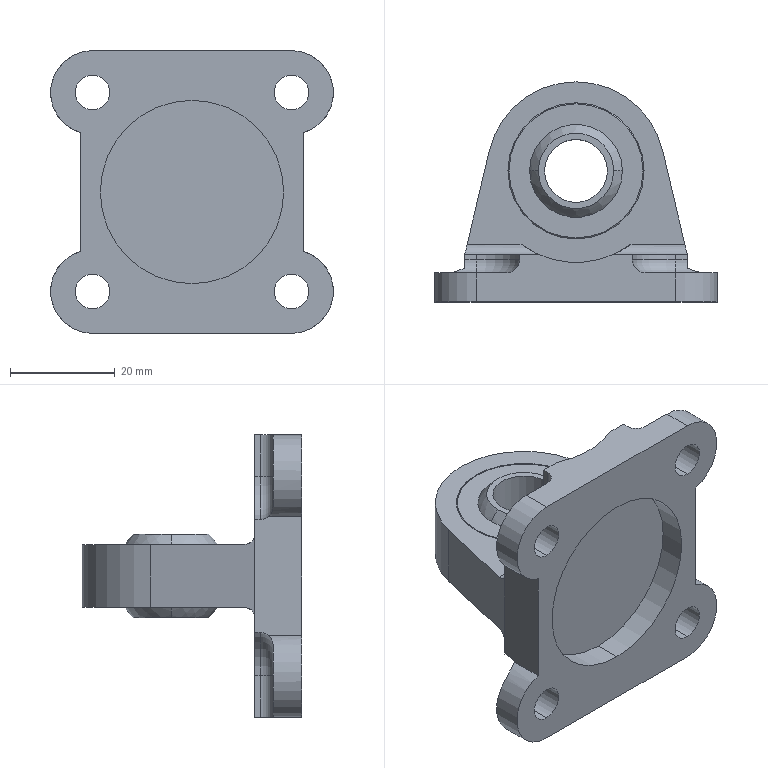Part | SolidWorks | features ICE 8, Fillet 3, HoleWzd 3, BaseBody 1 | 1 solid | 81 faces | box 54 x 42 x 54 mm | volume 25810 mm3 | cylinder 39 | plane 30 | cone 4 | spline 4 | torus 4 | commonest cylinder face diameters 5 x8 6.6 x8 4 x4 16 x4 16.5 x4 26 x4